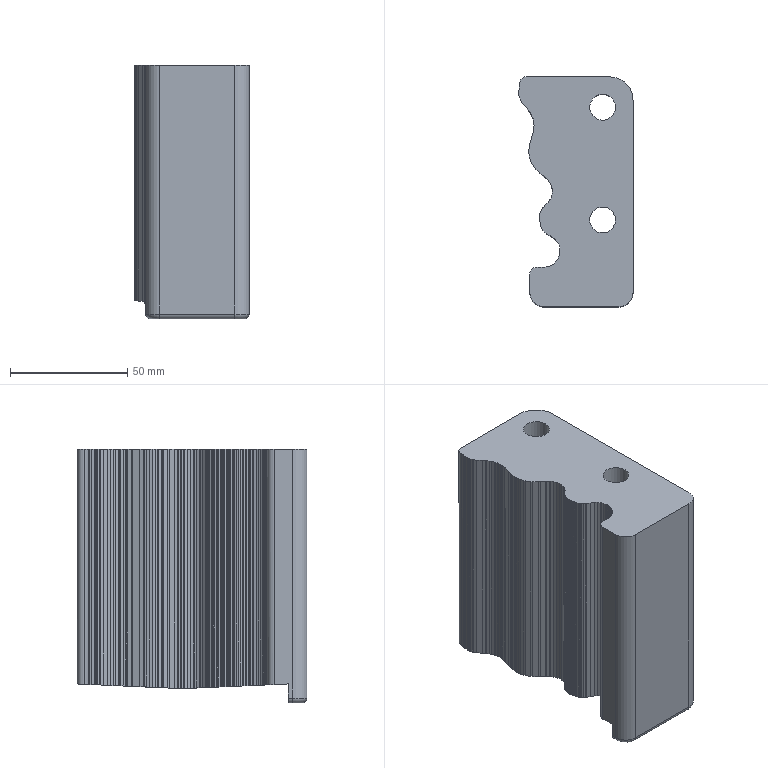Part | STEP file | PN_0028_id758_x_t | 1 solid | 249 faces | box 48.641 x 98 x 108 mm | volume 278628 mm3 | plane 176 | cylinder 68 | torus 4 | spline 1 | commonest cylinder face diameters 10 x51 12 x5 6 x4 4 x3 11 x2 17 x2